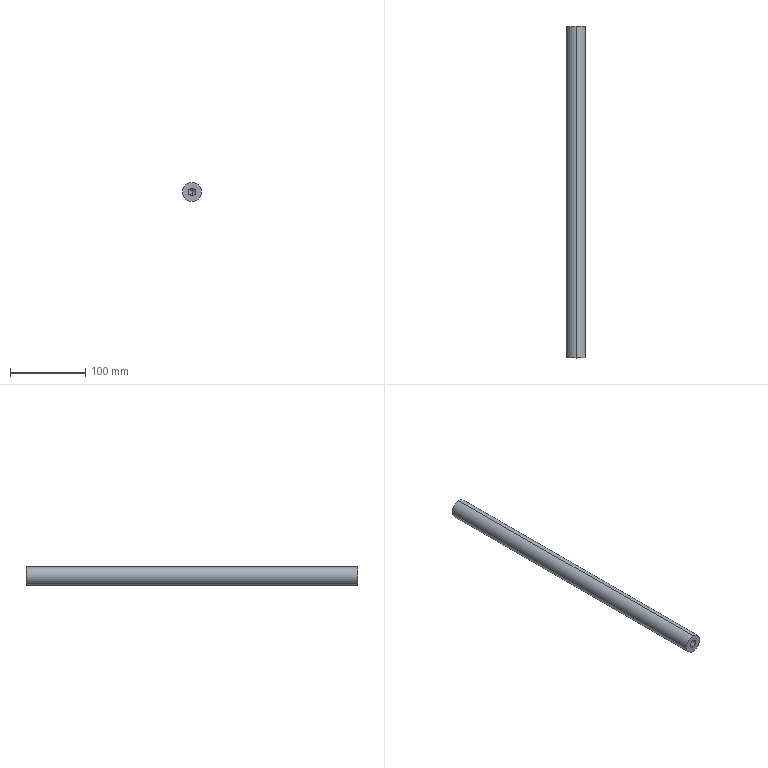Part | STEP file | slide shaft dia25x440 | 1 solid | 10 faces | box 25 x 440 x 25 mm | volume 213800 mm3 | cylinder 4 | cone 4 | plane 2 | commonest cylinder face diameters 10.2 x2 25 x2
STEP:
#1=CARTESIAN_POINT('',(0.,0.,0.));
#2=DIRECTION('',(0.,0.,1.));
#3=DIRECTION('',(1.,0.,0.));
#4=AXIS2_PLACEMENT_3D('',#1,#2,#3);
#5=CARTESIAN_POINT('',(0.,25.25,-5.1));
#6=VERTEX_POINT('',#5);
#7=CARTESIAN_POINT('',(0.,0.,-5.1));
#8=VERTEX_POINT('',#7);
#9=CARTESIAN_POINT('',(0.,-4.,-5.1));
#10=DIRECTION('',(0.,-1.,0.));
#11=VECTOR('',#10,1.);
#12=LINE('',#9,#11);
#13=CARTESIAN_POINT('',(0.,-4.,0.));
#14=DIRECTION('',(0.,-1.,0.));
#15=DIRECTION('',(0.,0.,-1.));
#16=AXIS2_PLACEMENT_3D('',#13,#14,#15);
#17=CYLINDRICAL_SURFACE('',#16,5.1);
#18=CARTESIAN_POINT('',(6.283,0.));
#19=DIRECTION('',(0.,1.));
#20=VECTOR('',#19,1.);
#21=LINE('',#18,#20);
#22=(GEOMETRIC_REPRESENTATION_CONTEXT(2)PARAMETRIC_REPRESENTATION_CONTEXT()REPRESENTATION_CONTEXT('',''));
#23=DEFINITIONAL_REPRESENTATION('',(#21),#22);
#24=PCURVE('',#17,#23);
#25=CARTESIAN_POINT('',(0.,-4.,0.));
#26=DIRECTION('',(0.,-1.,0.));
#27=DIRECTION('',(0.,0.,-1.));
#28=AXIS2_PLACEMENT_3D('',#25,#26,#27);
#29=CYLINDRICAL_SURFACE('',#28,5.1);
#30=CARTESIAN_POINT('',(0.,0.));
#31=DIRECTION('',(0.,1.));
#32=VECTOR('',#31,1.);
#33=LINE('',#30,#32);
#34=(GEOMETRIC_REPRESENTATION_CONTEXT(2)PARAMETRIC_REPRESENTATION_CONTEXT()REPRESENTATION_CONTEXT('',''));
#35=DEFINITIONAL_REPRESENTATION('',(#33),#34);
#36=PCURVE('',#29,#35);
#37=SURFACE_CURVE('',#12,(#24,#36),.PCURVE_S1.);
#38=EDGE_CURVE('',#6,#8,#37,.T.);
#39=ORIENTED_EDGE('',*,*,#38,.T.);
#40=CARTESIAN_POINT('',(0.,0.,5.1));
#41=VERTEX_POINT('',#40);
#42=CARTESIAN_POINT('',(0.,0.,0.));
#43=DIRECTION('',(0.,-1.,0.));
#44=DIRECTION('',(0.,0.,1.));
#45=AXIS2_PLACEMENT_3D('',#42,#43,#44);
#46=CIRCLE('',#45,5.1);
#47=CARTESIAN_POINT('',(3.142,-4.));
#48=DIRECTION('',(1.,0.));
#49=VECTOR('',#48,1.);
#50=LINE('',#47,#49);
#51=(GEOMETRIC_REPRESENTATION_CONTEXT(2)PARAMETRIC_REPRESENTATION_CONTEXT()REPRESENTATION_CONTEXT('',''));
#52=DEFINITIONAL_REPRESENTATION('',(#50),#51);
#53=PCURVE('',#17,#52);
#54=CARTESIAN_POINT('',(0.,0.,0.));
#55=DIRECTION('',(0.,1.,0.));
#56=DIRECTION('',(0.,0.,1.));
#57=AXIS2_PLACEMENT_3D('',#54,#55,#56);
#58=PLANE('',#57);
#59=CARTESIAN_POINT('',(5.1,0.));
#60=CARTESIAN_POINT('',(5.1,-8.833));
#61=CARTESIAN_POINT('',(-2.55,-4.417));
#62=CARTESIAN_POINT('',(-10.2,0.));
#63=CARTESIAN_POINT('',(-2.55,4.417));
#64=CARTESIAN_POINT('',(5.1,8.833));
#65=CARTESIAN_POINT('',(5.1,0.));
#66=(BOUNDED_CURVE()B_SPLINE_CURVE(2,(#59,#60,#61,#62,#63,#64,#65),.UNSPECIFIED.,.T.,.F.)B_SPLINE_CURVE_WITH_KNOTS((1,2,2,2,2,1),(-2.094,0.,2.094,4.189,6.283,8.378),.UNSPECIFIED.)CURVE()GEOMETRIC_REPRESENTATION_ITEM()RATIONAL_B_SPLINE_CURVE((1.,0.5,1.,0.5,1.,0.5,1.))REPRESENTATION_ITEM(''));
#67=(GEOMETRIC_REPRESENTATION_CONTEXT(2)PARAMETRIC_REPRESENTATION_CONTEXT()REPRESENTATION_CONTEXT('',''));
#68=DEFINITIONAL_REPRESENTATION('',(#66),#67);
#69=PCURVE('',#58,#68);
#70=SURFACE_CURVE('',#46,(#53,#69),.PCURVE_S1.);
#71=EDGE_CURVE('',#41,#8,#70,.T.);
#72=ORIENTED_EDGE('',*,*,#71,.F.);
#73=CARTESIAN_POINT('',(0.,25.25,5.1));
#74=VERTEX_POINT('',#73);
#75=CARTESIAN_POINT('',(0.,-4.,5.1));
#76=DIRECTION('',(0.,-1.,0.));
#77=VECTOR('',#76,1.);
#78=LINE('',#75,#77);
#79=CARTESIAN_POINT('',(3.142,0.));
#80=DIRECTION('',(0.,1.));
#81=VECTOR('',#80,1.);
#82=LINE('',#79,#81);
#83=(GEOMETRIC_REPRESENTATION_CONTEXT(2)PARAMETRIC_REPRESENTATION_CONTEXT()REPRESENTATION_CONTEXT('',''));
#84=DEFINITIONAL_REPRESENTATION('',(#82),#83);
#85=PCURVE('',#17,#84);
#86=CARTESIAN_POINT('',(3.142,0.));
#87=DIRECTION('',(0.,1.));
#88=VECTOR('',#87,1.);
#89=LINE('',#86,#88);
#90=(GEOMETRIC_REPRESENTATION_CONTEXT(2)PARAMETRIC_REPRESENTATION_CONTEXT()REPRESENTATION_CONTEXT('',''));
#91=DEFINITIONAL_REPRESENTATION('',(#89),#90);
#92=PCURVE('',#29,#91);
#93=SURFACE_CURVE('',#78,(#85,#92),.PCURVE_S1.);
#94=EDGE_CURVE('',#74,#41,#93,.T.);
#95=ORIENTED_EDGE('',*,*,#94,.F.);
#96=CARTESIAN_POINT('',(0.,25.25,0.));
#97=DIRECTION('',(0.,-1.,0.));
#98=DIRECTION('',(0.,0.,-1.));
#99=AXIS2_PLACEMENT_3D('',#96,#97,#98);
#100=CIRCLE('',#99,5.1);
#101=CARTESIAN_POINT('',(0.,-29.25));
#102=DIRECTION('',(1.,0.));
#103=VECTOR('',#102,1.);
#104=LINE('',#101,#103);
#105=(GEOMETRIC_REPRESENTATION_CONTEXT(2)PARAMETRIC_REPRESENTATION_CONTEXT()REPRESENTATION_CONTEXT('',''));
#106=DEFINITIONAL_REPRESENTATION('',(#104),#105);
#107=PCURVE('',#17,#106);
#108=CARTESIAN_POINT('',(0.,25.25,0.));
#109=DIRECTION('',(0.,-1.,0.));
#110=DIRECTION('',(0.,0.,-1.));
#111=AXIS2_PLACEMENT_3D('',#108,#109,#110);
#112=CONICAL_SURFACE('',#111,5.1,1.03);
#113=CARTESIAN_POINT('',(0.,0.));
#114=DIRECTION('',(1.,0.));
#115=VECTOR('',#114,1.);
#116=LINE('',#113,#115);
#117=(GEOMETRIC_REPRESENTATION_CONTEXT(2)PARAMETRIC_REPRESENTATION_CONTEXT()REPRESENTATION_CONTEXT('',''));
#118=DEFINITIONAL_REPRESENTATION('',(#116),#117);
#119=PCURVE('',#112,#118);
#120=SURFACE_CURVE('',#100,(#107,#119),.PCURVE_S1.);
#121=EDGE_CURVE('',#74,#6,#120,.T.);
#122=ORIENTED_EDGE('',*,*,#121,.T.);
#123=EDGE_LOOP('',(#39,#72,#95,#122));
#124=FACE_BOUND('',#123,.F.);
#125=ADVANCED_FACE('',(#124),#17,.F.);
#126=ORIENTED_EDGE('',*,*,#121,.F.);
#127=CARTESIAN_POINT('',(0.,28.314,0.));
#128=VERTEX_POINT('',#127);
#129=CARTESIAN_POINT('',(0.,25.25,5.1));
#130=DIRECTION('',(0.,-0.515,0.8572));
#131=VECTOR('',#130,1.);
#132=LINE('',#129,#131);
#133=CARTESIAN_POINT('',(3.142,0.));
#134=DIRECTION('',(0.,1.));
#135=VECTOR('',#134,1.);
#136=LINE('',#133,#135);
#137=(GEOMETRIC_REPRESENTATION_CONTEXT(2)PARAMETRIC_REPRESENTATION_CONTEXT()REPRESENTATION_CONTEXT('',''));
#138=DEFINITIONAL_REPRESENTATION('',(#136),#137);
#139=PCURVE('',#112,#138);
#140=CARTESIAN_POINT('',(0.,25.25,0.));
#141=DIRECTION('',(0.,-1.,0.));
#142=DIRECTION('',(0.,0.,-1.));
#143=AXIS2_PLACEMENT_3D('',#140,#141,#142);
#144=CONICAL_SURFACE('',#143,5.1,1.03);
#145=CARTESIAN_POINT('',(3.142,0.));
#146=DIRECTION('',(0.,1.));
#147=VECTOR('',#146,1.);
#148=LINE('',#145,#147);
#149=(GEOMETRIC_REPRESENTATION_CONTEXT(2)PARAMETRIC_REPRESENTATION_CONTEXT()REPRESENTATION_CONTEXT('',''));
#150=DEFINITIONAL_REPRESENTATION('',(#148),#149);
#151=PCURVE('',#144,#150);
#152=SURFACE_CURVE('',#132,(#139,#151),.PCURVE_S1.);
#153=EDGE_CURVE('',#128,#74,#152,.T.);
#154=ORIENTED_EDGE('',*,*,#153,.F.);
#155=CARTESIAN_POINT('',(0.,25.25,-5.1));
#156=DIRECTION('',(0.,-0.515,-0.8572));
#157=VECTOR('',#156,1.);
#158=LINE('',#155,#157);
#159=CARTESIAN_POINT('',(6.283,0.));
#160=DIRECTION('',(0.,1.));
#161=VECTOR('',#160,1.);
#162=LINE('',#159,#161);
#163=(GEOMETRIC_REPRESENTATION_CONTEXT(2)PARAMETRIC_REPRESENTATION_CONTEXT()REPRESENTATION_CONTEXT('',''));
#164=DEFINITIONAL_REPRESENTATION('',(#162),#163);
#165=PCURVE('',#112,#164);
#166=CARTESIAN_POINT('',(0.,0.));
#167=DIRECTION('',(0.,1.));
#168=VECTOR('',#167,1.);
#169=LINE('',#166,#168);
#170=(GEOMETRIC_REPRESENTATION_CONTEXT(2)PARAMETRIC_REPRESENTATION_CONTEXT()REPRESENTATION_CONTEXT('',''));
#171=DEFINITIONAL_REPRESENTATION('',(#169),#170);
#172=PCURVE('',#144,#171);
#173=SURFACE_CURVE('',#158,(#165,#172),.PCURVE_S1.);
#174=EDGE_CURVE('',#128,#6,#173,.T.);
#175=ORIENTED_EDGE('',*,*,#174,.T.);
#176=EDGE_LOOP('',(#126,#154,#175));
#177=FACE_BOUND('',#176,.F.);
#178=ADVANCED_FACE('',(#177),#112,.F.);
#179=CARTESIAN_POINT('',(0.,440.,11.5));
#180=VERTEX_POINT('',#179);
#181=CARTESIAN_POINT('',(0.,440.,-11.5));
#182=VERTEX_POINT('',#181);
#183=CARTESIAN_POINT('',(0.,440.,0.));
#184=DIRECTION('',(0.,1.,0.));
#185=DIRECTION('',(0.,0.,1.));
#186=AXIS2_PLACEMENT_3D('',#183,#184,#185);
#187=CIRCLE('',#186,11.5);
#188=CARTESIAN_POINT('',(0.,440.,0.));
#189=DIRECTION('',(0.,-1.,0.));
#190=DIRECTION('',(0.,0.,-1.));
#191=AXIS2_PLACEMENT_3D('',#188,#189,#190);
#192=CONICAL_SURFACE('',#191,11.5,0.7854);
#193=CARTESIAN_POINT('',(3.142,0.));
#194=DIRECTION('',(-1.,0.));
#195=VECTOR('',#194,1.);
#196=LINE('',#193,#195);
#197=(GEOMETRIC_REPRESENTATION_CONTEXT(2)PARAMETRIC_REPRESENTATION_CONTEXT()REPRESENTATION_CONTEXT('',''));
#198=DEFINITIONAL_REPRESENTATION('',(#196),#197);
#199=PCURVE('',#192,#198);
#200=CARTESIAN_POINT('',(0.,440.,0.));
#201=DIRECTION('',(0.,1.,0.));
#202=DIRECTION('',(0.,0.,1.));
#203=AXIS2_PLACEMENT_3D('',#200,#201,#202);
#204=PLANE('',#203);
#205=CARTESIAN_POINT('',(0.,0.));
#206=DIRECTION('',(1.,0.));
#207=AXIS2_PLACEMENT_2D('',#205,#206);
#208=CIRCLE('',#207,11.5);
#209=(GEOMETRIC_REPRESENTATION_CONTEXT(2)PARAMETRIC_REPRESENTATION_CONTEXT()REPRESENTATION_CONTEXT('',''));
#210=DEFINITIONAL_REPRESENTATION('',(#208),#209);
#211=PCURVE('',#204,#210);
#212=SURFACE_CURVE('',#187,(#199,#211),.PCURVE_S1.);
#213=EDGE_CURVE('',#180,#182,#212,.T.);
#214=ORIENTED_EDGE('',*,*,#213,.F.);
#215=CARTESIAN_POINT('',(0.,439.,12.5));
#216=VERTEX_POINT('',#215);
#217=CARTESIAN_POINT('',(0.,440.,11.5));
#218=DIRECTION('',(0.,-0.7071,0.7071));
#219=VECTOR('',#218,1.);
#220=LINE('',#217,#219);
#221=CARTESIAN_POINT('',(3.142,0.));
#222=DIRECTION('',(0.,1.));
#223=VECTOR('',#222,1.);
#224=LINE('',#221,#223);
#225=(GEOMETRIC_REPRESENTATION_CONTEXT(2)PARAMETRIC_REPRESENTATION_CONTEXT()REPRESENTATION_CONTEXT('',''));
#226=DEFINITIONAL_REPRESENTATION('',(#224),#225);
#227=PCURVE('',#192,#226);
#228=CARTESIAN_POINT('',(0.,440.,0.));
#229=DIRECTION('',(0.,-1.,0.));
#230=DIRECTION('',(0.,0.,-1.));
#231=AXIS2_PLACEMENT_3D('',#228,#229,#230);
#232=CONICAL_SURFACE('',#231,11.5,0.7854);
#233=CARTESIAN_POINT('',(3.142,0.));
#234=DIRECTION('',(0.,1.));
#235=VECTOR('',#234,1.);
#236=LINE('',#233,#235);
#237=(GEOMETRIC_REPRESENTATION_CONTEXT(2)PARAMETRIC_REPRESENTATION_CONTEXT()REPRESENTATION_CONTEXT('',''));
#238=DEFINITIONAL_REPRESENTATION('',(#236),#237);
#239=PCURVE('',#232,#238);
#240=SURFACE_CURVE('',#220,(#227,#239),.PCURVE_S1.);
#241=EDGE_CURVE('',#180,#216,#240,.T.);
#242=ORIENTED_EDGE('',*,*,#241,.T.);
#243=CARTESIAN_POINT('',(0.,439.,-12.5));
#244=VERTEX_POINT('',#243);
#245=CARTESIAN_POINT('',(0.,439.,0.));
#246=DIRECTION('',(0.,-1.,0.));
#247=DIRECTION('',(0.,0.,1.));
#248=AXIS2_PLACEMENT_3D('',#245,#246,#247);
#249=CIRCLE('',#248,12.5);
#250=CARTESIAN_POINT('',(-3.142,1.));
#251=DIRECTION('',(1.,0.));
#252=VECTOR('',#251,1.);
#253=LINE('',#250,#252);
#254=(GEOMETRIC_REPRESENTATION_CONTEXT(2)PARAMETRIC_REPRESENTATION_CONTEXT()REPRESENTATION_CONTEXT('',''));
#255=DEFINITIONAL_REPRESENTATION('',(#253),#254);
#256=PCURVE('',#192,#255);
#257=CARTESIAN_POINT('',(0.,440.,0.));
#258=DIRECTION('',(0.,-1.,0.));
#259=DIRECTION('',(0.,0.,-1.));
#260=AXIS2_PLACEMENT_3D('',#257,#258,#259);
#261=CYLINDRICAL_SURFACE('',#260,12.5);
#262=CARTESIAN_POINT('',(-3.142,1.));
#263=DIRECTION('',(1.,0.));
#264=VECTOR('',#263,1.);
#265=LINE('',#262,#264);
#266=(GEOMETRIC_REPRESENTATION_CONTEXT(2)PARAMETRIC_REPRESENTATION_CONTEXT()REPRESENTATION_CONTEXT('',''));
#267=DEFINITIONAL_REPRESENTATION('',(#265),#266);
#268=PCURVE('',#261,#267);
#269=SURFACE_CURVE('',#249,(#256,#268),.PCURVE_S1.);
#270=EDGE_CURVE('',#244,#216,#269,.T.);
#271=ORIENTED_EDGE('',*,*,#270,.F.);
#272=CARTESIAN_POINT('',(0.,440.,-11.5));
#273=DIRECTION('',(0.,-0.7071,-0.7071));
#274=VECTOR('',#273,1.);
#275=LINE('',#272,#274);
#276=CARTESIAN_POINT('',(0.,0.));
#277=DIRECTION('',(0.,1.));
#278=VECTOR('',#277,1.);
#279=LINE('',#276,#278);
#280=(GEOMETRIC_REPRESENTATION_CONTEXT(2)PARAMETRIC_REPRESENTATION_CONTEXT()REPRESENTATION_CONTEXT('',''));
#281=DEFINITIONAL_REPRESENTATION('',(#279),#280);
#282=PCURVE('',#192,#281);
#283=CARTESIAN_POINT('',(6.283,0.));
#284=DIRECTION('',(0.,1.));
#285=VECTOR('',#284,1.);
#286=LINE('',#283,#285);
#287=(GEOMETRIC_REPRESENTATION_CONTEXT(2)PARAMETRIC_REPRESENTATION_CONTEXT()REPRESENTATION_CONTEXT('',''));
#288=DEFINITIONAL_REPRESENTATION('',(#286),#287);
#289=PCURVE('',#232,#288);
#290=SURFACE_CURVE('',#275,(#282,#289),.PCURVE_S1.);
#291=EDGE_CURVE('',#182,#244,#290,.T.);
#292=ORIENTED_EDGE('',*,*,#291,.F.);
#293=EDGE_LOOP('',(#214,#242,#271,#292));
#294=FACE_BOUND('',#293,.T.);
#295=ADVANCED_FACE('',(#294),#192,.T.);
#296=ORIENTED_EDGE('',*,*,#270,.T.);
#297=CARTESIAN_POINT('',(0.,0.,12.5));
#298=VERTEX_POINT('',#297);
#299=CARTESIAN_POINT('',(0.,440.,12.5));
#300=DIRECTION('',(0.,-1.,0.));
#301=VECTOR('',#300,1.);
#302=LINE('',#299,#301);
#303=CARTESIAN_POINT('',(3.142,0.));
#304=DIRECTION('',(0.,1.));
#305=VECTOR('',#304,1.);
#306=LINE('',#303,#305);
#307=(GEOMETRIC_REPRESENTATION_CONTEXT(2)PARAMETRIC_REPRESENTATION_CONTEXT()REPRESENTATION_CONTEXT('',''));
#308=DEFINITIONAL_REPRESENTATION('',(#306),#307);
#309=PCURVE('',#261,#308);
#310=CARTESIAN_POINT('',(0.,440.,0.));
#311=DIRECTION('',(0.,-1.,0.));
#312=DIRECTION('',(0.,0.,-1.));
#313=AXIS2_PLACEMENT_3D('',#310,#311,#312);
#314=CYLINDRICAL_SURFACE('',#313,12.5);
#315=CARTESIAN_POINT('',(3.142,0.));
#316=DIRECTION('',(0.,1.));
#317=VECTOR('',#316,1.);
#318=LINE('',#315,#317);
#319=(GEOMETRIC_REPRESENTATION_CONTEXT(2)PARAMETRIC_REPRESENTATION_CONTEXT()REPRESENTATION_CONTEXT('',''));
#320=DEFINITIONAL_REPRESENTATION('',(#318),#319);
#321=PCURVE('',#314,#320);
#322=SURFACE_CURVE('',#302,(#309,#321),.PCURVE_S1.);
#323=EDGE_CURVE('',#216,#298,#322,.T.);
#324=ORIENTED_EDGE('',*,*,#323,.T.);
#325=CARTESIAN_POINT('',(0.,0.,-12.5));
#326=VERTEX_POINT('',#325);
#327=CARTESIAN_POINT('',(0.,0.,0.));
#328=DIRECTION('',(0.,1.,0.));
#329=DIRECTION('',(0.,0.,1.));
#330=AXIS2_PLACEMENT_3D('',#327,#328,#329);
#331=CIRCLE('',#330,12.5);
#332=CARTESIAN_POINT('',(3.142,440.));
#333=DIRECTION('',(-1.,0.));
#334=VECTOR('',#333,1.);
#335=LINE('',#332,#334);
#336=(GEOMETRIC_REPRESENTATION_CONTEXT(2)PARAMETRIC_REPRESENTATION_CONTEXT()REPRESENTATION_CONTEXT('',''));
#337=DEFINITIONAL_REPRESENTATION('',(#335),#336);
#338=PCURVE('',#261,#337);
#339=CARTESIAN_POINT('',(0.,0.));
#340=DIRECTION('',(1.,0.));
#341=AXIS2_PLACEMENT_2D('',#339,#340);
#342=CIRCLE('',#341,12.5);
#343=(GEOMETRIC_REPRESENTATION_CONTEXT(2)PARAMETRIC_REPRESENTATION_CONTEXT()REPRESENTATION_CONTEXT('',''));
#344=DEFINITIONAL_REPRESENTATION('',(#342),#343);
#345=PCURVE('',#58,#344);
#346=SURFACE_CURVE('',#331,(#338,#345),.PCURVE_S1.);
#347=EDGE_CURVE('',#298,#326,#346,.T.);
#348=ORIENTED_EDGE('',*,*,#347,.T.);
#349=CARTESIAN_POINT('',(0.,440.,-12.5));
#350=DIRECTION('',(0.,-1.,0.));
#351=VECTOR('',#350,1.);
#352=LINE('',#349,#351);
#353=CARTESIAN_POINT('',(0.,0.));
#354=DIRECTION('',(0.,1.));
#355=VECTOR('',#354,1.);
#356=LINE('',#353,#355);
#357=(GEOMETRIC_REPRESENTATION_CONTEXT(2)PARAMETRIC_REPRESENTATION_CONTEXT()REPRESENTATION_CONTEXT('',''));
#358=DEFINITIONAL_REPRESENTATION('',(#356),#357);
#359=PCURVE('',#261,#358);
#360=CARTESIAN_POINT('',(6.283,0.));
#361=DIRECTION('',(0.,1.));
#362=VECTOR('',#361,1.);
#363=LINE('',#360,#362);
#364=(GEOMETRIC_REPRESENTATION_CONTEXT(2)PARAMETRIC_REPRESENTATION_CONTEXT()REPRESENTATION_CONTEXT('',''));
#365=DEFINITIONAL_REPRESENTATION('',(#363),#364);
#366=PCURVE('',#314,#365);
#367=SURFACE_CURVE('',#352,(#359,#366),.PCURVE_S1.);
#368=EDGE_CURVE('',#244,#326,#367,.T.);
#369=ORIENTED_EDGE('',*,*,#368,.F.);
#370=EDGE_LOOP('',(#296,#324,#348,#369));
#371=FACE_BOUND('',#370,.T.);
#372=ADVANCED_FACE('',(#371),#261,.T.);
#373=CARTESIAN_POINT('',(0.,0.,0.));
#374=DIRECTION('',(0.,1.,0.));
#375=DIRECTION('',(0.,0.,1.));
#376=AXIS2_PLACEMENT_3D('',#373,#374,#375);
#377=CIRCLE('',#376,12.5);
#378=CARTESIAN_POINT('',(0.,0.));
#379=DIRECTION('',(1.,0.));
#380=AXIS2_PLACEMENT_2D('',#378,#379);
#381=CIRCLE('',#380,12.5);
#382=(GEOMETRIC_REPRESENTATION_CONTEXT(2)PARAMETRIC_REPRESENTATION_CONTEXT()REPRESENTATION_CONTEXT('',''));
#383=DEFINITIONAL_REPRESENTATION('',(#381),#382);
#384=PCURVE('',#58,#383);
#385=CARTESIAN_POINT('',(9.425,440.));
#386=DIRECTION('',(-1.,0.));
#387=VECTOR('',#386,1.);
#388=LINE('',#385,#387);
#389=(GEOMETRIC_REPRESENTATION_CONTEXT(2)PARAMETRIC_REPRESENTATION_CONTEXT()REPRESENTATION_CONTEXT('',''));
#390=DEFINITIONAL_REPRESENTATION('',(#388),#389);
#391=PCURVE('',#314,#390);
#392=SURFACE_CURVE('',#377,(#384,#391),.PCURVE_S1.);
#393=EDGE_CURVE('',#326,#298,#392,.T.);
#394=ORIENTED_EDGE('',*,*,#393,.F.);
#395=ORIENTED_EDGE('',*,*,#347,.F.);
#396=EDGE_LOOP('',(#394,#395));
#397=FACE_BOUND('',#396,.T.);
#398=CARTESIAN_POINT('',(0.,0.,0.));
#399=DIRECTION('',(0.,-1.,0.));
#400=DIRECTION('',(0.,0.,1.));
#401=AXIS2_PLACEMENT_3D('',#398,#399,#400);
#402=CIRCLE('',#401,5.1);
#403=CARTESIAN_POINT('',(5.1,0.));
#404=CARTESIAN_POINT('',(5.1,-8.833));
#405=CARTESIAN_POINT('',(-2.55,-4.417));
#406=CARTESIAN_POINT('',(-10.2,0.));
#407=CARTESIAN_POINT('',(-2.55,4.417));
#408=CARTESIAN_POINT('',(5.1,8.833));
#409=CARTESIAN_POINT('',(5.1,0.));
#410=(BOUNDED_CURVE()B_SPLINE_CURVE(2,(#403,#404,#405,#406,#407,#408,#409),.UNSPECIFIED.,.T.,.F.)B_SPLINE_CURVE_WITH_KNOTS((1,2,2,2,2,1),(-2.094,0.,2.094,4.189,6.283,8.378),.UNSPECIFIED.)CURVE()GEOMETRIC_REPRESENTATION_ITEM()RATIONAL_B_SPLINE_CURVE((1.,0.5,1.,0.5,1.,0.5,1.))REPRESENTATION_ITEM(''));
#411=(GEOMETRIC_REPRESENTATION_CONTEXT(2)PARAMETRIC_REPRESENTATION_CONTEXT()REPRESENTATION_CONTEXT('',''));
#412=DEFINITIONAL_REPRESENTATION('',(#410),#411);
#413=PCURVE('',#58,#412);
#414=CARTESIAN_POINT('',(-3.142,-4.));
#415=DIRECTION('',(1.,0.));
#416=VECTOR('',#415,1.);
#417=LINE('',#414,#416);
#418=(GEOMETRIC_REPRESENTATION_CONTEXT(2)PARAMETRIC_REPRESENTATION_CONTEXT()REPRESENTATION_CONTEXT('',''));
#419=DEFINITIONAL_REPRESENTATION('',(#417),#418);
#420=PCURVE('',#29,#419);
#421=SURFACE_CURVE('',#402,(#413,#420),.PCURVE_S1.);
#422=EDGE_CURVE('',#8,#41,#421,.T.);
#423=ORIENTED_EDGE('',*,*,#422,.F.);
#424=ORIENTED_EDGE('',*,*,#71,.F.);
#425=EDGE_LOOP('',(#423,#424));
#426=FACE_BOUND('',#425,.T.);
#427=ADVANCED_FACE('',(#397,#426),#58,.F.);
#428=ORIENTED_EDGE('',*,*,#323,.F.);
#429=CARTESIAN_POINT('',(0.,439.,0.));
#430=DIRECTION('',(0.,-1.,0.));
#431=DIRECTION('',(0.,0.,1.));
#432=AXIS2_PLACEMENT_3D('',#429,#430,#431);
#433=CIRCLE('',#432,12.5);
#434=CARTESIAN_POINT('',(3.142,1.));
#435=DIRECTION('',(1.,0.));
#436=VECTOR('',#435,1.);
#437=LINE('',#434,#436);
#438=(GEOMETRIC_REPRESENTATION_CONTEXT(2)PARAMETRIC_REPRESENTATION_CONTEXT()REPRESENTATION_CONTEXT('',''));
#439=DEFINITIONAL_REPRESENTATION('',(#437),#438);
#440=PCURVE('',#314,#439);
#441=CARTESIAN_POINT('',(3.142,1.));
#442=DIRECTION('',(1.,0.));
#443=VECTOR('',#442,1.);
#444=LINE('',#441,#443);
#445=(GEOMETRIC_REPRESENTATION_CONTEXT(2)PARAMETRIC_REPRESENTATION_CONTEXT()REPRESENTATION_CONTEXT('',''));
#446=DEFINITIONAL_REPRESENTATION('',(#444),#445);
#447=PCURVE('',#232,#446);
#448=SURFACE_CURVE('',#433,(#440,#447),.PCURVE_S1.);
#449=EDGE_CURVE('',#216,#244,#448,.T.);
#450=ORIENTED_EDGE('',*,*,#449,.T.);
#451=ORIENTED_EDGE('',*,*,#368,.T.);
#452=ORIENTED_EDGE('',*,*,#393,.T.);
#453=EDGE_LOOP('',(#428,#450,#451,#452));
#454=FACE_BOUND('',#453,.T.);
#455=ADVANCED_FACE('',(#454),#314,.T.);
#456=CARTESIAN_POINT('',(0.,440.,0.));
#457=DIRECTION('',(0.,1.,0.));
#458=DIRECTION('',(0.,0.,1.));
#459=AXIS2_PLACEMENT_3D('',#456,#457,#458);
#460=CIRCLE('',#459,11.5);
#461=CARTESIAN_POINT('',(0.,0.));
#462=DIRECTION('',(1.,0.));
#463=AXIS2_PLACEMENT_2D('',#461,#462);
#464=CIRCLE('',#463,11.5);
#465=(GEOMETRIC_REPRESENTATION_CONTEXT(2)PARAMETRIC_REPRESENTATION_CONTEXT()REPRESENTATION_CONTEXT('',''));
#466=DEFINITIONAL_REPRESENTATION('',(#464),#465);
#467=PCURVE('',#204,#466);
#468=CARTESIAN_POINT('',(9.425,0.));
#469=DIRECTION('',(-1.,0.));
#470=VECTOR('',#469,1.);
#471=LINE('',#468,#470);
#472=(GEOMETRIC_REPRESENTATION_CONTEXT(2)PARAMETRIC_REPRESENTATION_CONTEXT()REPRESENTATION_CONTEXT('',''));
#473=DEFINITIONAL_REPRESENTATION('',(#471),#472);
#474=PCURVE('',#232,#473);
#475=SURFACE_CURVE('',#460,(#467,#474),.PCURVE_S1.);
#476=EDGE_CURVE('',#182,#180,#475,.T.);
#477=ORIENTED_EDGE('',*,*,#476,.T.);
#478=ORIENTED_EDGE('',*,*,#213,.T.);
#479=EDGE_LOOP('',(#477,#478));
#480=FACE_BOUND('',#479,.T.);
#481=ADVANCED_FACE('',(#480),#204,.T.);
#482=ORIENTED_EDGE('',*,*,#241,.F.);
#483=ORIENTED_EDGE('',*,*,#476,.F.);
#484=ORIENTED_EDGE('',*,*,#291,.T.);
#485=ORIENTED_EDGE('',*,*,#449,.F.);
#486=EDGE_LOOP('',(#482,#483,#484,#485));
#487=FACE_BOUND('',#486,.T.);
#488=ADVANCED_FACE('',(#487),#232,.T.);
#489=CARTESIAN_POINT('',(0.,25.25,0.));
#490=DIRECTION('',(0.,-1.,0.));
#491=DIRECTION('',(0.,0.,-1.));
#492=AXIS2_PLACEMENT_3D('',#489,#490,#491);
#493=CIRCLE('',#492,5.1);
#494=CARTESIAN_POINT('',(0.,0.));
#495=DIRECTION('',(1.,0.));
#496=VECTOR('',#495,1.);
#497=LINE('',#494,#496);
#498=(GEOMETRIC_REPRESENTATION_CONTEXT(2)PARAMETRIC_REPRESENTATION_CONTEXT()REPRESENTATION_CONTEXT('',''));
#499=DEFINITIONAL_REPRESENTATION('',(#497),#498);
#500=PCURVE('',#144,#499);
#501=CARTESIAN_POINT('',(0.,-29.25));
#502=DIRECTION('',(1.,0.));
#503=VECTOR('',#502,1.);
#504=LINE('',#501,#503);
#505=(GEOMETRIC_REPRESENTATION_CONTEXT(2)PARAMETRIC_REPRESENTATION_CONTEXT()REPRESENTATION_CONTEXT('',''));
#506=DEFINITIONAL_REPRESENTATION('',(#504),#505);
#507=PCURVE('',#29,#506);
#508=SURFACE_CURVE('',#493,(#500,#507),.PCURVE_S1.);
#509=EDGE_CURVE('',#6,#74,#508,.T.);
#510=ORIENTED_EDGE('',*,*,#509,.F.);
#511=ORIENTED_EDGE('',*,*,#174,.F.);
#512=ORIENTED_EDGE('',*,*,#153,.T.);
#513=EDGE_LOOP('',(#510,#511,#512));
#514=FACE_BOUND('',#513,.F.);
#515=ADVANCED_FACE('',(#514),#144,.F.);
#516=ORIENTED_EDGE('',*,*,#422,.F.);
#517=ORIENTED_EDGE('',*,*,#38,.F.);
#518=ORIENTED_EDGE('',*,*,#509,.T.);
#519=ORIENTED_EDGE('',*,*,#94,.T.);
#520=EDGE_LOOP('',(#516,#517,#518,#519));
#521=FACE_BOUND('',#520,.F.);
#522=ADVANCED_FACE('',(#521),#29,.F.);
#523=CLOSED_SHELL('',(#125,#178,#295,#372,#427,#455,#481,#488,#515,#522));
#524=MANIFOLD_SOLID_BREP('',#523);
#525=(LENGTH_UNIT()NAMED_UNIT(*)SI_UNIT(.MILLI.,.METRE.));
#526=UNCERTAINTY_MEASURE_WITH_UNIT(LENGTH_MEASURE(0.0000001),#525,'','');
#527=(NAMED_UNIT(*)PLANE_ANGLE_UNIT()SI_UNIT($,.RADIAN.));
#528=(NAMED_UNIT(*)SI_UNIT($,.STERADIAN.)SOLID_ANGLE_UNIT());
#529=(GEOMETRIC_REPRESENTATION_CONTEXT(3)GLOBAL_UNCERTAINTY_ASSIGNED_CONTEXT((#526))GLOBAL_UNIT_ASSIGNED_CONTEXT((#525,#527,#528))REPRESENTATION_CONTEXT('',''));
#530=ADVANCED_BREP_SHAPE_REPRESENTATION('',(#4,#524),#529);